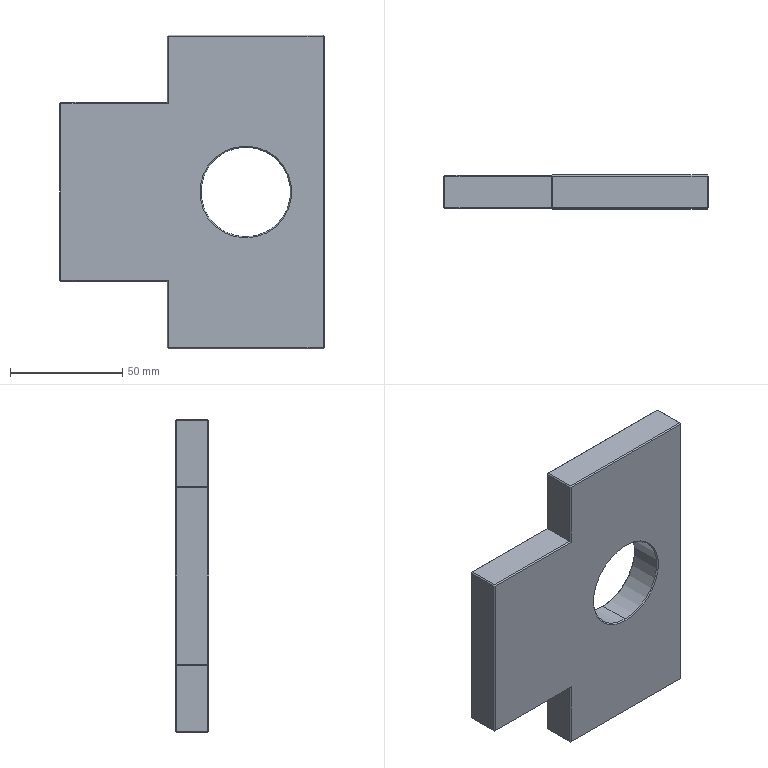Part | SolidWorks | features Chamfer 1, Extrusion 1 | 1 solid | 50 faces | box 118 x 15 x 140 mm | volume 185579 mm3 | plane 44 | cone 4 | cylinder 2 | commonest cylinder face diameters 40 x2
STEP:
#1=CARTESIAN_POINT('',(-35.,14.5,-20.));
#2=VERTEX_POINT('',#1);
#3=CARTESIAN_POINT('',(-35.,14.5,20.));
#4=VERTEX_POINT('',#3);
#5=CARTESIAN_POINT('',(-35.,14.5,0.));
#6=DIRECTION('',(0.,1.,0.));
#7=DIRECTION('',(0.,0.,-1.));
#8=AXIS2_PLACEMENT_3D('',#5,#6,#7);
#9=CIRCLE('',#8,20.);
#10=EDGE_CURVE('',#2,#4,#9,.T.);
#11=ORIENTED_EDGE('',*,*,#10,.F.);
#12=CARTESIAN_POINT('',(-35.,15.,-20.5));
#13=VERTEX_POINT('',#12);
#14=CARTESIAN_POINT('',(-35.,14.5,-20.));
#15=DIRECTION('',(0.,0.7071,-0.7071));
#16=VECTOR('',#15,1000.);
#17=LINE('',#14,#16);
#18=EDGE_CURVE('',#2,#13,#17,.T.);
#19=ORIENTED_EDGE('',*,*,#18,.T.);
#20=CARTESIAN_POINT('',(-35.,15.,20.5));
#21=VERTEX_POINT('',#20);
#22=CARTESIAN_POINT('',(-35.,15.,0.));
#23=DIRECTION('',(0.,-1.,0.));
#24=DIRECTION('',(0.,0.,-1.));
#25=AXIS2_PLACEMENT_3D('',#22,#23,#24);
#26=CIRCLE('',#25,20.5);
#27=EDGE_CURVE('',#21,#13,#26,.T.);
#28=ORIENTED_EDGE('',*,*,#27,.F.);
#29=CARTESIAN_POINT('',(-35.,14.5,20.));
#30=DIRECTION('',(0.,0.7071,0.7071));
#31=VECTOR('',#30,1000.);
#32=LINE('',#29,#31);
#33=EDGE_CURVE('',#4,#21,#32,.T.);
#34=ORIENTED_EDGE('',*,*,#33,.F.);
#35=EDGE_LOOP('',(#11,#19,#28,#34));
#36=FACE_OUTER_BOUND('',#35,.T.);
#37=CARTESIAN_POINT('',(-35.,14.5,0.));
#38=DIRECTION('',(0.,1.,0.));
#39=DIRECTION('',(0.,0.,1.));
#40=AXIS2_PLACEMENT_3D('',#37,#38,#39);
#41=CONICAL_SURFACE('',#40,20.,0.7854);
#42=ADVANCED_FACE('',(#36),#41,.F.);
#43=CARTESIAN_POINT('',(-35.,0.5,20.));
#44=VERTEX_POINT('',#43);
#45=CARTESIAN_POINT('',(-35.,0.5,-20.));
#46=VERTEX_POINT('',#45);
#47=CARTESIAN_POINT('',(-35.,0.5,0.));
#48=DIRECTION('',(0.,-1.,0.));
#49=DIRECTION('',(0.,0.,-1.));
#50=AXIS2_PLACEMENT_3D('',#47,#48,#49);
#51=CIRCLE('',#50,20.);
#52=EDGE_CURVE('',#44,#46,#51,.T.);
#53=ORIENTED_EDGE('',*,*,#52,.F.);
#54=CARTESIAN_POINT('',(-35.,0.,20.5));
#55=VERTEX_POINT('',#54);
#56=CARTESIAN_POINT('',(-35.,0.,20.5));
#57=DIRECTION('',(0.,-0.7071,0.7071));
#58=VECTOR('',#57,1000.);
#59=LINE('',#56,#58);
#60=EDGE_CURVE('',#44,#55,#59,.T.);
#61=ORIENTED_EDGE('',*,*,#60,.T.);
#62=CARTESIAN_POINT('',(-35.,0.,-20.5));
#63=VERTEX_POINT('',#62);
#64=CARTESIAN_POINT('',(-35.,0.,0.));
#65=DIRECTION('',(0.,1.,0.));
#66=DIRECTION('',(0.,0.,-1.));
#67=AXIS2_PLACEMENT_3D('',#64,#65,#66);
#68=CIRCLE('',#67,20.5);
#69=EDGE_CURVE('',#63,#55,#68,.T.);
#70=ORIENTED_EDGE('',*,*,#69,.F.);
#71=CARTESIAN_POINT('',(-35.,0.,-20.5));
#72=DIRECTION('',(0.,-0.7071,-0.7071));
#73=VECTOR('',#72,1000.);
#74=LINE('',#71,#73);
#75=EDGE_CURVE('',#46,#63,#74,.T.);
#76=ORIENTED_EDGE('',*,*,#75,.F.);
#77=EDGE_LOOP('',(#53,#61,#70,#76));
#78=FACE_OUTER_BOUND('',#77,.T.);
#79=CARTESIAN_POINT('',(-35.,0.,0.));
#80=DIRECTION('',(0.,-1.,0.));
#81=DIRECTION('',(0.,0.,-1.));
#82=AXIS2_PLACEMENT_3D('',#79,#80,#81);
#83=CONICAL_SURFACE('',#82,20.5,0.7854);
#84=ADVANCED_FACE('',(#78),#83,.F.);
#85=ORIENTED_EDGE('',*,*,#10,.T.);
#86=CARTESIAN_POINT('',(-35.,15.,20.));
#87=DIRECTION('',(0.,-1.,0.));
#88=VECTOR('',#87,1000.);
#89=LINE('',#86,#88);
#90=EDGE_CURVE('',#4,#44,#89,.T.);
#91=ORIENTED_EDGE('',*,*,#90,.T.);
#92=ORIENTED_EDGE('',*,*,#52,.T.);
#93=CARTESIAN_POINT('',(-35.,15.,-20.));
#94=DIRECTION('',(0.,-1.,0.));
#95=VECTOR('',#94,1000.);
#96=LINE('',#93,#95);
#97=EDGE_CURVE('',#2,#46,#96,.T.);
#98=ORIENTED_EDGE('',*,*,#97,.F.);
#99=EDGE_LOOP('',(#85,#91,#92,#98));
#100=FACE_OUTER_BOUND('',#99,.T.);
#101=CARTESIAN_POINT('',(-35.,15.,0.));
#102=DIRECTION('',(0.,-1.,0.));
#103=DIRECTION('',(0.,0.,-1.));
#104=AXIS2_PLACEMENT_3D('',#101,#102,#103);
#105=CYLINDRICAL_SURFACE('',#104,20.);
#106=ADVANCED_FACE('',(#100),#105,.F.);
#107=CARTESIAN_POINT('',(-117.5,15.,39.5));
#108=VERTEX_POINT('',#107);
#109=CARTESIAN_POINT('',(-69.5,15.,39.5));
#110=VERTEX_POINT('',#109);
#111=CARTESIAN_POINT('',(0.,15.,39.5));
#112=DIRECTION('',(1.,0.,0.));
#113=VECTOR('',#112,1000.);
#114=LINE('',#111,#113);
#115=EDGE_CURVE('',#108,#110,#114,.T.);
#116=ORIENTED_EDGE('',*,*,#115,.T.);
#117=CARTESIAN_POINT('',(-69.5,15.,69.5));
#118=VERTEX_POINT('',#117);
#119=CARTESIAN_POINT('',(-69.5,15.,0.));
#120=DIRECTION('',(0.,0.,1.));
#121=VECTOR('',#120,1000.);
#122=LINE('',#119,#121);
#123=EDGE_CURVE('',#110,#118,#122,.T.);
#124=ORIENTED_EDGE('',*,*,#123,.T.);
#125=CARTESIAN_POINT('',(-0.5,15.,69.5));
#126=VERTEX_POINT('',#125);
#127=CARTESIAN_POINT('',(0.,15.,69.5));
#128=DIRECTION('',(1.,0.,0.));
#129=VECTOR('',#128,1000.);
#130=LINE('',#127,#129);
#131=EDGE_CURVE('',#118,#126,#130,.T.);
#132=ORIENTED_EDGE('',*,*,#131,.T.);
#133=CARTESIAN_POINT('',(-0.5,15.,-69.5));
#134=VERTEX_POINT('',#133);
#135=CARTESIAN_POINT('',(-0.5,15.,0.));
#136=DIRECTION('',(0.,0.,-1.));
#137=VECTOR('',#136,1000.);
#138=LINE('',#135,#137);
#139=EDGE_CURVE('',#126,#134,#138,.T.);
#140=ORIENTED_EDGE('',*,*,#139,.T.);
#141=CARTESIAN_POINT('',(-69.5,15.,-69.5));
#142=VERTEX_POINT('',#141);
#143=CARTESIAN_POINT('',(0.,15.,-69.5));
#144=DIRECTION('',(-1.,0.,0.));
#145=VECTOR('',#144,1000.);
#146=LINE('',#143,#145);
#147=EDGE_CURVE('',#134,#142,#146,.T.);
#148=ORIENTED_EDGE('',*,*,#147,.T.);
#149=CARTESIAN_POINT('',(-69.5,15.,-39.5));
#150=VERTEX_POINT('',#149);
#151=CARTESIAN_POINT('',(-69.5,15.,0.));
#152=DIRECTION('',(0.,0.,1.));
#153=VECTOR('',#152,1000.);
#154=LINE('',#151,#153);
#155=EDGE_CURVE('',#142,#150,#154,.T.);
#156=ORIENTED_EDGE('',*,*,#155,.T.);
#157=CARTESIAN_POINT('',(-117.5,15.,-39.5));
#158=VERTEX_POINT('',#157);
#159=CARTESIAN_POINT('',(0.,15.,-39.5));
#160=DIRECTION('',(-1.,0.,0.));
#161=VECTOR('',#160,1000.);
#162=LINE('',#159,#161);
#163=EDGE_CURVE('',#150,#158,#162,.T.);
#164=ORIENTED_EDGE('',*,*,#163,.T.);
#165=CARTESIAN_POINT('',(-117.5,15.,0.));
#166=DIRECTION('',(0.,0.,1.));
#167=VECTOR('',#166,1000.);
#168=LINE('',#165,#167);
#169=EDGE_CURVE('',#158,#108,#168,.T.);
#170=ORIENTED_EDGE('',*,*,#169,.T.);
#171=EDGE_LOOP('',(#116,#124,#132,#140,#148,#156,#164,#170));
#172=FACE_OUTER_BOUND('',#171,.T.);
#173=ORIENTED_EDGE('',*,*,#27,.T.);
#174=CARTESIAN_POINT('',(-35.,15.,0.));
#175=DIRECTION('',(0.,-1.,0.));
#176=DIRECTION('',(0.,0.,-1.));
#177=AXIS2_PLACEMENT_3D('',#174,#175,#176);
#178=CIRCLE('',#177,20.5);
#179=EDGE_CURVE('',#13,#21,#178,.T.);
#180=ORIENTED_EDGE('',*,*,#179,.T.);
#181=EDGE_LOOP('',(#173,#180));
#182=FACE_BOUND('',#181,.T.);
#183=CARTESIAN_POINT('',(0.,15.,0.));
#184=DIRECTION('',(0.,-1.,0.));
#185=DIRECTION('',(0.,0.,-1.));
#186=AXIS2_PLACEMENT_3D('',#183,#184,#185);
#187=PLANE('',#186);
#188=ADVANCED_FACE('',(#172,#182),#187,.F.);
#189=ORIENTED_EDGE('',*,*,#69,.T.);
#190=CARTESIAN_POINT('',(-35.,0.,0.));
#191=DIRECTION('',(0.,1.,0.));
#192=DIRECTION('',(0.,0.,-1.));
#193=AXIS2_PLACEMENT_3D('',#190,#191,#192);
#194=CIRCLE('',#193,20.5);
#195=EDGE_CURVE('',#55,#63,#194,.T.);
#196=ORIENTED_EDGE('',*,*,#195,.T.);
#197=EDGE_LOOP('',(#189,#196));
#198=FACE_BOUND('',#197,.T.);
#199=CARTESIAN_POINT('',(-0.5,0.,69.5));
#200=VERTEX_POINT('',#199);
#201=CARTESIAN_POINT('',(-69.5,0.,69.5));
#202=VERTEX_POINT('',#201);
#203=CARTESIAN_POINT('',(-70.,0.,69.5));
#204=DIRECTION('',(-1.,0.,0.));
#205=VECTOR('',#204,1000.);
#206=LINE('',#203,#205);
#207=EDGE_CURVE('',#200,#202,#206,.T.);
#208=ORIENTED_EDGE('',*,*,#207,.T.);
#209=CARTESIAN_POINT('',(-69.5,0.,39.5));
#210=VERTEX_POINT('',#209);
#211=CARTESIAN_POINT('',(-69.5,0.,40.));
#212=DIRECTION('',(0.,0.,-1.));
#213=VECTOR('',#212,1000.);
#214=LINE('',#211,#213);
#215=EDGE_CURVE('',#202,#210,#214,.T.);
#216=ORIENTED_EDGE('',*,*,#215,.T.);
#217=CARTESIAN_POINT('',(-117.5,0.,39.5));
#218=VERTEX_POINT('',#217);
#219=CARTESIAN_POINT('',(-118.,0.,39.5));
#220=DIRECTION('',(-1.,0.,0.));
#221=VECTOR('',#220,1000.);
#222=LINE('',#219,#221);
#223=EDGE_CURVE('',#210,#218,#222,.T.);
#224=ORIENTED_EDGE('',*,*,#223,.T.);
#225=CARTESIAN_POINT('',(-117.5,0.,-39.5));
#226=VERTEX_POINT('',#225);
#227=CARTESIAN_POINT('',(-117.5,0.,-40.));
#228=DIRECTION('',(0.,0.,-1.));
#229=VECTOR('',#228,1000.);
#230=LINE('',#227,#229);
#231=EDGE_CURVE('',#218,#226,#230,.T.);
#232=ORIENTED_EDGE('',*,*,#231,.T.);
#233=CARTESIAN_POINT('',(-69.5,0.,-39.5));
#234=VERTEX_POINT('',#233);
#235=CARTESIAN_POINT('',(-70.,0.,-39.5));
#236=DIRECTION('',(1.,0.,0.));
#237=VECTOR('',#236,1000.);
#238=LINE('',#235,#237);
#239=EDGE_CURVE('',#226,#234,#238,.T.);
#240=ORIENTED_EDGE('',*,*,#239,.T.);
#241=CARTESIAN_POINT('',(-69.5,0.,-69.5));
#242=VERTEX_POINT('',#241);
#243=CARTESIAN_POINT('',(-69.5,0.,-70.));
#244=DIRECTION('',(0.,0.,-1.));
#245=VECTOR('',#244,1000.);
#246=LINE('',#243,#245);
#247=EDGE_CURVE('',#234,#242,#246,.T.);
#248=ORIENTED_EDGE('',*,*,#247,.T.);
#249=CARTESIAN_POINT('',(-0.5,0.,-69.5));
#250=VERTEX_POINT('',#249);
#251=CARTESIAN_POINT('',(0.,0.,-69.5));
#252=DIRECTION('',(1.,0.,0.));
#253=VECTOR('',#252,1000.);
#254=LINE('',#251,#253);
#255=EDGE_CURVE('',#242,#250,#254,.T.);
#256=ORIENTED_EDGE('',*,*,#255,.T.);
#257=CARTESIAN_POINT('',(-0.5,0.,70.));
#258=DIRECTION('',(0.,0.,1.));
#259=VECTOR('',#258,1000.);
#260=LINE('',#257,#259);
#261=EDGE_CURVE('',#250,#200,#260,.T.);
#262=ORIENTED_EDGE('',*,*,#261,.T.);
#263=EDGE_LOOP('',(#208,#216,#224,#232,#240,#248,#256,#262));
#264=FACE_OUTER_BOUND('',#263,.T.);
#265=CARTESIAN_POINT('',(0.,0.,0.));
#266=DIRECTION('',(0.,-1.,0.));
#267=DIRECTION('',(0.,0.,-1.));
#268=AXIS2_PLACEMENT_3D('',#265,#266,#267);
#269=PLANE('',#268);
#270=ADVANCED_FACE('',(#198,#264),#269,.T.);
#271=CARTESIAN_POINT('',(-0.5,0.5,70.));
#272=VERTEX_POINT('',#271);
#273=CARTESIAN_POINT('',(-0.5,14.5,70.));
#274=VERTEX_POINT('',#273);
#275=CARTESIAN_POINT('',(-0.5,15.,70.));
#276=DIRECTION('',(0.,1.,0.));
#277=VECTOR('',#276,1000.);
#278=LINE('',#275,#277);
#279=EDGE_CURVE('',#272,#274,#278,.T.);
#280=ORIENTED_EDGE('',*,*,#279,.T.);
#281=CARTESIAN_POINT('',(-69.5,14.5,70.));
#282=VERTEX_POINT('',#281);
#283=CARTESIAN_POINT('',(0.,14.5,70.));
#284=DIRECTION('',(-1.,0.,0.));
#285=VECTOR('',#284,1000.);
#286=LINE('',#283,#285);
#287=EDGE_CURVE('',#274,#282,#286,.T.);
#288=ORIENTED_EDGE('',*,*,#287,.T.);
#289=CARTESIAN_POINT('',(-69.5,0.5,70.));
#290=VERTEX_POINT('',#289);
#291=CARTESIAN_POINT('',(-69.5,15.,70.));
#292=DIRECTION('',(0.,-1.,0.));
#293=VECTOR('',#292,1000.);
#294=LINE('',#291,#293);
#295=EDGE_CURVE('',#282,#290,#294,.T.);
#296=ORIENTED_EDGE('',*,*,#295,.T.);
#297=CARTESIAN_POINT('',(0.,0.5,70.));
#298=DIRECTION('',(1.,0.,0.));
#299=VECTOR('',#298,1000.);
#300=LINE('',#297,#299);
#301=EDGE_CURVE('',#290,#272,#300,.T.);
#302=ORIENTED_EDGE('',*,*,#301,.T.);
#303=EDGE_LOOP('',(#280,#288,#296,#302));
#304=FACE_OUTER_BOUND('',#303,.T.);
#305=CARTESIAN_POINT('',(0.,15.,70.));
#306=DIRECTION('',(0.,0.,-1.));
#307=DIRECTION('',(-1.,0.,0.));
#308=AXIS2_PLACEMENT_3D('',#305,#306,#307);
#309=PLANE('',#308);
#310=ADVANCED_FACE('',(#304),#309,.F.);
#311=CARTESIAN_POINT('',(0.,0.5,-69.5));
#312=VERTEX_POINT('',#311);
#313=CARTESIAN_POINT('',(0.,14.5,-69.5));
#314=VERTEX_POINT('',#313);
#315=CARTESIAN_POINT('',(0.,15.,-69.5));
#316=DIRECTION('',(0.,1.,0.));
#317=VECTOR('',#316,1000.);
#318=LINE('',#315,#317);
#319=EDGE_CURVE('',#312,#314,#318,.T.);
#320=ORIENTED_EDGE('',*,*,#319,.T.);
#321=CARTESIAN_POINT('',(0.,14.5,69.5));
#322=VERTEX_POINT('',#321);
#323=CARTESIAN_POINT('',(0.,14.5,-70.));
#324=DIRECTION('',(0.,0.,1.));
#325=VECTOR('',#324,1000.);
#326=LINE('',#323,#325);
#327=EDGE_CURVE('',#314,#322,#326,.T.);
#328=ORIENTED_EDGE('',*,*,#327,.T.);
#329=CARTESIAN_POINT('',(0.,0.5,69.5));
#330=VERTEX_POINT('',#329);
#331=CARTESIAN_POINT('',(0.,15.,69.5));
#332=DIRECTION('',(0.,-1.,0.));
#333=VECTOR('',#332,1000.);
#334=LINE('',#331,#333);
#335=EDGE_CURVE('',#322,#330,#334,.T.);
#336=ORIENTED_EDGE('',*,*,#335,.T.);
#337=CARTESIAN_POINT('',(0.,0.5,-70.));
#338=DIRECTION('',(0.,0.,-1.));
#339=VECTOR('',#338,1000.);
#340=LINE('',#337,#339);
#341=EDGE_CURVE('',#330,#312,#340,.T.);
#342=ORIENTED_EDGE('',*,*,#341,.T.);
#343=EDGE_LOOP('',(#320,#328,#336,#342));
#344=FACE_OUTER_BOUND('',#343,.T.);
#345=CARTESIAN_POINT('',(0.,15.,-70.));
#346=DIRECTION('',(-1.,0.,0.));
#347=DIRECTION('',(0.,0.,1.));
#348=AXIS2_PLACEMENT_3D('',#345,#346,#347);
#349=PLANE('',#348);
#350=ADVANCED_FACE('',(#344),#349,.F.);
#351=CARTESIAN_POINT('',(-69.5,14.5,-70.));
#352=VERTEX_POINT('',#351);
#353=CARTESIAN_POINT('',(-0.5,14.5,-70.));
#354=VERTEX_POINT('',#353);
#355=CARTESIAN_POINT('',(-70.,14.5,-70.));
#356=DIRECTION('',(1.,0.,0.));
#357=VECTOR('',#356,1000.);
#358=LINE('',#355,#357);
#359=EDGE_CURVE('',#352,#354,#358,.T.);
#360=ORIENTED_EDGE('',*,*,#359,.T.);
#361=CARTESIAN_POINT('',(-0.5,0.5,-70.));
#362=VERTEX_POINT('',#361);
#363=CARTESIAN_POINT('',(-0.5,15.,-70.));
#364=DIRECTION('',(0.,-1.,0.));
#365=VECTOR('',#364,1000.);
#366=LINE('',#363,#365);
#367=EDGE_CURVE('',#354,#362,#366,.T.);
#368=ORIENTED_EDGE('',*,*,#367,.T.);
#369=CARTESIAN_POINT('',(-69.5,0.5,-70.));
#370=VERTEX_POINT('',#369);
#371=CARTESIAN_POINT('',(-70.,0.5,-70.));
#372=DIRECTION('',(-1.,0.,0.));
#373=VECTOR('',#372,1000.);
#374=LINE('',#371,#373);
#375=EDGE_CURVE('',#362,#370,#374,.T.);
#376=ORIENTED_EDGE('',*,*,#375,.T.);
#377=CARTESIAN_POINT('',(-69.5,15.,-70.));
#378=DIRECTION('',(0.,1.,0.));
#379=VECTOR('',#378,1000.);
#380=LINE('',#377,#379);
#381=EDGE_CURVE('',#370,#352,#380,.T.);
#382=ORIENTED_EDGE('',*,*,#381,.T.);
#383=EDGE_LOOP('',(#360,#368,#376,#382));
#384=FACE_OUTER_BOUND('',#383,.T.);
#385=CARTESIAN_POINT('',(-70.,15.,-70.));
#386=DIRECTION('',(0.,0.,1.));
#387=DIRECTION('',(1.,0.,0.));
#388=AXIS2_PLACEMENT_3D('',#385,#386,#387);
#389=PLANE('',#388);
#390=ADVANCED_FACE('',(#384),#389,.F.);
#391=CARTESIAN_POINT('',(-70.,14.5,-40.));
#392=VERTEX_POINT('',#391);
#393=CARTESIAN_POINT('',(-70.,0.5,-40.));
#394=VERTEX_POINT('',#393);
#395=CARTESIAN_POINT('',(-70.,15.,-40.));
#396=DIRECTION('',(0.,-1.,0.));
#397=VECTOR('',#396,1000.);
#398=LINE('',#395,#397);
#399=EDGE_CURVE('',#392,#394,#398,.T.);
#400=ORIENTED_EDGE('',*,*,#399,.F.);
#401=CARTESIAN_POINT('',(-70.,14.5,-69.5));
#402=VERTEX_POINT('',#401);
#403=CARTESIAN_POINT('',(-70.,14.5,-40.));
#404=DIRECTION('',(0.,0.,-1.));
#405=VECTOR('',#404,1000.);
#406=LINE('',#403,#405);
#407=EDGE_CURVE('',#392,#402,#406,.T.);
#408=ORIENTED_EDGE('',*,*,#407,.T.);
#409=CARTESIAN_POINT('',(-70.,0.5,-69.5));
#410=VERTEX_POINT('',#409);
#411=CARTESIAN_POINT('',(-70.,15.,-69.5));
#412=DIRECTION('',(0.,-1.,0.));
#413=VECTOR('',#412,1000.);
#414=LINE('',#411,#413);
#415=EDGE_CURVE('',#402,#410,#414,.T.);
#416=ORIENTED_EDGE('',*,*,#415,.T.);
#417=CARTESIAN_POINT('',(-70.,0.5,-40.));
#418=DIRECTION('',(0.,0.,1.));
#419=VECTOR('',#418,1000.);
#420=LINE('',#417,#419);
#421=EDGE_CURVE('',#410,#394,#420,.T.);
#422=ORIENTED_EDGE('',*,*,#421,.T.);
#423=EDGE_LOOP('',(#400,#408,#416,#422));
#424=FACE_OUTER_BOUND('',#423,.T.);
#425=CARTESIAN_POINT('',(-70.,15.,-40.));
#426=DIRECTION('',(1.,0.,0.));
#427=DIRECTION('',(0.,0.,-1.));
#428=AXIS2_PLACEMENT_3D('',#425,#426,#427);
#429=PLANE('',#428);
#430=ADVANCED_FACE('',(#424),#429,.F.);
#431=CARTESIAN_POINT('',(-117.5,0.5,-40.));
#432=VERTEX_POINT('',#431);
#433=CARTESIAN_POINT('',(-117.5,14.5,-40.));
#434=VERTEX_POINT('',#433);
#435=CARTESIAN_POINT('',(-117.5,15.,-40.));
#436=DIRECTION('',(0.,1.,0.));
#437=VECTOR('',#436,1000.);
#438=LINE('',#435,#437);
#439=EDGE_CURVE('',#432,#434,#438,.T.);
#440=ORIENTED_EDGE('',*,*,#439,.T.);
#441=CARTESIAN_POINT('',(-118.,14.5,-40.));
#442=DIRECTION('',(1.,0.,0.));
#443=VECTOR('',#442,1000.);
#444=LINE('',#441,#443);
#445=EDGE_CURVE('',#434,#392,#444,.T.);
#446=ORIENTED_EDGE('',*,*,#445,.T.);
#447=ORIENTED_EDGE('',*,*,#399,.T.);
#448=CARTESIAN_POINT('',(-118.,0.5,-40.));
#449=DIRECTION('',(-1.,0.,0.));
#450=VECTOR('',#449,1000.);
#451=LINE('',#448,#450);
#452=EDGE_CURVE('',#394,#432,#451,.T.);
#453=ORIENTED_EDGE('',*,*,#452,.T.);
#454=EDGE_LOOP('',(#440,#446,#447,#453));
#455=FACE_OUTER_BOUND('',#454,.T.);
#456=CARTESIAN_POINT('',(-118.,15.,-40.));
#457=DIRECTION('',(0.,0.,1.));
#458=DIRECTION('',(1.,0.,0.));
#459=AXIS2_PLACEMENT_3D('',#456,#457,#458);
#460=PLANE('',#459);
#461=ADVANCED_FACE('',(#455),#460,.F.);
#462=CARTESIAN_POINT('',(-118.,0.5,39.5));
#463=VERTEX_POINT('',#462);
#464=CARTESIAN_POINT('',(-118.,14.5,39.5));
#465=VERTEX_POINT('',#464);
#466=CARTESIAN_POINT('',(-118.,15.,39.5));
#467=DIRECTION('',(0.,1.,0.));
#468=VECTOR('',#467,1000.);
#469=LINE('',#466,#468);
#470=EDGE_CURVE('',#463,#465,#469,.T.);
#471=ORIENTED_EDGE('',*,*,#470,.T.);
#472=CARTESIAN_POINT('',(-118.,14.5,-39.5));
#473=VERTEX_POINT('',#472);
#474=CARTESIAN_POINT('',(-118.,14.5,40.));
#475=DIRECTION('',(0.,0.,-1.));
#476=VECTOR('',#475,1000.);
#477=LINE('',#474,#476);
#478=EDGE_CURVE('',#465,#473,#477,.T.);
#479=ORIENTED_EDGE('',*,*,#478,.T.);
#480=CARTESIAN_POINT('',(-118.,0.5,-39.5));
#481=VERTEX_POINT('',#480);
#482=CARTESIAN_POINT('',(-118.,15.,-39.5));
#483=DIRECTION('',(0.,-1.,0.));
#484=VECTOR('',#483,1000.);
#485=LINE('',#482,#484);
#486=EDGE_CURVE('',#473,#481,#485,.T.);
#487=ORIENTED_EDGE('',*,*,#486,.T.);
#488=CARTESIAN_POINT('',(-118.,0.5,40.));
#489=DIRECTION('',(0.,0.,1.));
#490=VECTOR('',#489,1000.);
#491=LINE('',#488,#490);
#492=EDGE_CURVE('',#481,#463,#491,.T.);
#493=ORIENTED_EDGE('',*,*,#492,.T.);
#494=EDGE_LOOP('',(#471,#479,#487,#493));
#495=FACE_OUTER_BOUND('',#494,.T.);
#496=CARTESIAN_POINT('',(-118.,15.,40.));
#497=DIRECTION('',(1.,0.,0.));
#498=DIRECTION('',(0.,0.,-1.));
#499=AXIS2_PLACEMENT_3D('',#496,#497,#498);
#500=PLANE('',#499);
#501=ADVANCED_FACE('',(#495),#500,.F.);
#502=CARTESIAN_POINT('',(-70.,14.5,40.));
#503=VERTEX_POINT('',#502);
#504=CARTESIAN_POINT('',(-70.,0.5,40.));
#505=VERTEX_POINT('',#504);
#506=CARTESIAN_POINT('',(-70.,15.,40.));
#507=DIRECTION('',(0.,-1.,0.));
#508=VECTOR('',#507,1000.);
#509=LINE('',#506,#508);
#510=EDGE_CURVE('',#503,#505,#509,.T.);
#511=ORIENTED_EDGE('',*,*,#510,.F.);
#512=CARTESIAN_POINT('',(-117.5,14.5,40.));
#513=VERTEX_POINT('',#512);
#514=CARTESIAN_POINT('',(-70.,14.5,40.));
#515=DIRECTION('',(-1.,0.,0.));
#516=VECTOR('',#515,1000.);
#517=LINE('',#514,#516);
#518=EDGE_CURVE('',#503,#513,#517,.T.);
#519=ORIENTED_EDGE('',*,*,#518,.T.);
#520=CARTESIAN_POINT('',(-117.5,0.5,40.));
#521=VERTEX_POINT('',#520);
#522=CARTESIAN_POINT('',(-117.5,15.,40.));
#523=DIRECTION('',(0.,-1.,0.));
#524=VECTOR('',#523,1000.);
#525=LINE('',#522,#524);
#526=EDGE_CURVE('',#513,#521,#525,.T.);
#527=ORIENTED_EDGE('',*,*,#526,.T.);
#528=CARTESIAN_POINT('',(-70.,0.5,40.));
#529=DIRECTION('',(1.,0.,0.));
#530=VECTOR('',#529,1000.);
#531=LINE('',#528,#530);
#532=EDGE_CURVE('',#521,#505,#531,.T.);
#533=ORIENTED_EDGE('',*,*,#532,.T.);
#534=EDGE_LOOP('',(#511,#519,#527,#533));
#535=FACE_OUTER_BOUND('',#534,.T.);
#536=CARTESIAN_POINT('',(-70.,15.,40.));
#537=DIRECTION('',(0.,0.,-1.));
#538=DIRECTION('',(-1.,0.,0.));
#539=AXIS2_PLACEMENT_3D('',#536,#537,#538);
#540=PLANE('',#539);
#541=ADVANCED_FACE('',(#535),#540,.F.);
#542=CARTESIAN_POINT('',(-70.,0.5,69.5));
#543=VERTEX_POINT('',#542);
#544=CARTESIAN_POINT('',(-70.,14.5,69.5));
#545=VERTEX_POINT('',#544);
#546=CARTESIAN_POINT('',(-70.,15.,69.5));
#547=DIRECTION('',(0.,1.,0.));
#548=VECTOR('',#547,1000.);
#549=LINE('',#546,#548);
#550=EDGE_CURVE('',#543,#545,#549,.T.);
#551=ORIENTED_EDGE('',*,*,#550,.T.);
#552=CARTESIAN_POINT('',(-70.,14.5,70.));
#553=DIRECTION('',(0.,0.,-1.));
#554=VECTOR('',#553,1000.);
#555=LINE('',#552,#554);
#556=EDGE_CURVE('',#545,#503,#555,.T.);
#557=ORIENTED_EDGE('',*,*,#556,.T.);
#558=ORIENTED_EDGE('',*,*,#510,.T.);
#559=CARTESIAN_POINT('',(-70.,0.5,70.));
#560=DIRECTION('',(0.,0.,1.));
#561=VECTOR('',#560,1000.);
#562=LINE('',#559,#561);
#563=EDGE_CURVE('',#505,#543,#562,.T.);
#564=ORIENTED_EDGE('',*,*,#563,.T.);
#565=EDGE_LOOP('',(#551,#557,#558,#564));
#566=FACE_OUTER_BOUND('',#565,.T.);
#567=CARTESIAN_POINT('',(-70.,15.,70.));
#568=DIRECTION('',(1.,0.,0.));
#569=DIRECTION('',(0.,0.,-1.));
#570=AXIS2_PLACEMENT_3D('',#567,#568,#569);
#571=PLANE('',#570);
#572=ADVANCED_FACE('',(#566),#571,.F.);
#573=ORIENTED_EDGE('',*,*,#90,.F.);
#574=CARTESIAN_POINT('',(-35.,14.5,0.));
#575=DIRECTION('',(0.,1.,0.));
#576=DIRECTION('',(0.,0.,-1.));
#577=AXIS2_PLACEMENT_3D('',#574,#575,#576);
#578=CIRCLE('',#577,20.);
#579=EDGE_CURVE('',#4,#2,#578,.T.);
#580=ORIENTED_EDGE('',*,*,#579,.T.);
#581=ORIENTED_EDGE('',*,*,#97,.T.);
#582=CARTESIAN_POINT('',(-35.,0.5,0.));
#583=DIRECTION('',(0.,-1.,0.));
#584=DIRECTION('',(0.,0.,-1.));
#585=AXIS2_PLACEMENT_3D('',#582,#583,#584);
#586=CIRCLE('',#585,20.);
#587=EDGE_CURVE('',#46,#44,#586,.T.);
#588=ORIENTED_EDGE('',*,*,#587,.T.);
#589=EDGE_LOOP('',(#573,#580,#581,#588));
#590=FACE_OUTER_BOUND('',#589,.T.);
#591=CARTESIAN_POINT('',(-35.,15.,0.));
#592=DIRECTION('',(0.,-1.,0.));
#593=DIRECTION('',(0.,0.,-1.));
#594=AXIS2_PLACEMENT_3D('',#591,#592,#593);
#595=CYLINDRICAL_SURFACE('',#594,20.);
#596=ADVANCED_FACE('',(#590),#595,.F.);
#597=ORIENTED_EDGE('',*,*,#60,.F.);
#598=ORIENTED_EDGE('',*,*,#587,.F.);
#599=ORIENTED_EDGE('',*,*,#75,.T.);
#600=ORIENTED_EDGE('',*,*,#195,.F.);
#601=EDGE_LOOP('',(#597,#598,#599,#600));
#602=FACE_OUTER_BOUND('',#601,.T.);
#603=CARTESIAN_POINT('',(-35.,0.,0.));
#604=DIRECTION('',(0.,-1.,0.));
#605=DIRECTION('',(0.,0.,-1.));
#606=AXIS2_PLACEMENT_3D('',#603,#604,#605);
#607=CONICAL_SURFACE('',#606,20.5,0.7854);
#608=ADVANCED_FACE('',(#602),#607,.F.);
#609=CARTESIAN_POINT('',(-118.,14.5,39.5));
#610=DIRECTION('',(0.7071,0.,0.7071));
#611=VECTOR('',#610,1000.);
#612=LINE('',#609,#611);
#613=EDGE_CURVE('',#465,#513,#612,.T.);
#614=ORIENTED_EDGE('',*,*,#613,.F.);
#615=ORIENTED_EDGE('',*,*,#470,.F.);
#616=CARTESIAN_POINT('',(-117.5,0.5,40.));
#617=DIRECTION('',(-0.7071,0.,-0.7071));
#618=VECTOR('',#617,1000.);
#619=LINE('',#616,#618);
#620=EDGE_CURVE('',#521,#463,#619,.T.);
#621=ORIENTED_EDGE('',*,*,#620,.F.);
#622=ORIENTED_EDGE('',*,*,#526,.F.);
#623=EDGE_LOOP('',(#614,#615,#621,#622));
#624=FACE_OUTER_BOUND('',#623,.T.);
#625=CARTESIAN_POINT('',(-117.5,15.,40.));
#626=DIRECTION('',(0.7071,0.,-0.7071));
#627=DIRECTION('',(0.,-1.,0.));
#628=AXIS2_PLACEMENT_3D('',#625,#626,#627);
#629=PLANE('',#628);
#630=ADVANCED_FACE('',(#624),#629,.F.);
#631=CARTESIAN_POINT('',(-118.,14.5,39.5));
#632=DIRECTION('',(0.7071,0.7071,0.));
#633=VECTOR('',#632,1000.);
#634=LINE('',#631,#633);
#635=EDGE_CURVE('',#465,#108,#634,.T.);
#636=ORIENTED_EDGE('',*,*,#635,.F.);
#637=ORIENTED_EDGE('',*,*,#613,.T.);
#638=CARTESIAN_POINT('',(-117.5,14.75,39.75));
#639=DIRECTION('',(0.,-0.7071,0.7071));
#640=VECTOR('',#639,1000.);
#641=LINE('',#638,#640);
#642=EDGE_CURVE('',#108,#513,#641,.T.);
#643=ORIENTED_EDGE('',*,*,#642,.F.);
#644=EDGE_LOOP('',(#636,#637,#643));
#645=FACE_OUTER_BOUND('',#644,.T.);
#646=CARTESIAN_POINT('',(-118.,14.5,39.5));
#647=DIRECTION('',(-0.5774,0.5774,0.5774));
#648=DIRECTION('',(0.7071,0.,0.7071));
#649=AXIS2_PLACEMENT_3D('',#646,#647,#648);
#650=PLANE('',#649);
#651=ADVANCED_FACE('',(#645),#650,.T.);
#652=CARTESIAN_POINT('',(-117.5,0.5,40.));
#653=DIRECTION('',(0.,-0.7071,-0.7071));
#654=VECTOR('',#653,1000.);
#655=LINE('',#652,#654);
#656=EDGE_CURVE('',#521,#218,#655,.T.);
#657=ORIENTED_EDGE('',*,*,#656,.F.);
#658=ORIENTED_EDGE('',*,*,#620,.T.);
#659=CARTESIAN_POINT('',(-117.75,0.25,39.5));
#660=DIRECTION('',(-0.7071,0.7071,0.));
#661=VECTOR('',#660,1000.);
#662=LINE('',#659,#661);
#663=EDGE_CURVE('',#218,#463,#662,.T.);
#664=ORIENTED_EDGE('',*,*,#663,.F.);
#665=EDGE_LOOP('',(#657,#658,#664));
#666=FACE_OUTER_BOUND('',#665,.T.);
#667=CARTESIAN_POINT('',(-117.5,0.5,40.));
#668=DIRECTION('',(-0.5774,-0.5774,0.5774));
#669=DIRECTION('',(0.7071,0.,0.7071));
#670=AXIS2_PLACEMENT_3D('',#667,#668,#669);
#671=PLANE('',#670);
#672=ADVANCED_FACE('',(#666),#671,.T.);
#673=ORIENTED_EDGE('',*,*,#642,.T.);
#674=ORIENTED_EDGE('',*,*,#518,.F.);
#675=CARTESIAN_POINT('',(-56.333,28.167,26.333));
#676=DIRECTION('',(-0.5774,-0.5774,0.5774));
#677=VECTOR('',#676,1000.);
#678=LINE('',#675,#677);
#679=EDGE_CURVE('',#110,#503,#678,.T.);
#680=ORIENTED_EDGE('',*,*,#679,.F.);
#681=ORIENTED_EDGE('',*,*,#115,.F.);
#682=EDGE_LOOP('',(#673,#674,#680,#681));
#683=FACE_OUTER_BOUND('',#682,.T.);
#684=CARTESIAN_POINT('',(0.,15.,39.5));
#685=DIRECTION('',(0.,-0.7071,-0.7071));
#686=DIRECTION('',(1.,0.,0.));
#687=AXIS2_PLACEMENT_3D('',#684,#685,#686);
#688=PLANE('',#687);
#689=ADVANCED_FACE('',(#683),#688,.F.);
#690=ORIENTED_EDGE('',*,*,#635,.T.);
#691=ORIENTED_EDGE('',*,*,#169,.F.);
#692=CARTESIAN_POINT('',(-117.75,14.75,-39.5));
#693=DIRECTION('',(0.7071,0.7071,0.));
#694=VECTOR('',#693,1000.);
#695=LINE('',#692,#694);
#696=EDGE_CURVE('',#473,#158,#695,.T.);
#697=ORIENTED_EDGE('',*,*,#696,.F.);
#698=ORIENTED_EDGE('',*,*,#478,.F.);
#699=EDGE_LOOP('',(#690,#691,#697,#698));
#700=FACE_OUTER_BOUND('',#699,.T.);
#701=CARTESIAN_POINT('',(-117.5,15.,0.));
#702=DIRECTION('',(0.7071,-0.7071,0.));
#703=DIRECTION('',(0.,0.,1.));
#704=AXIS2_PLACEMENT_3D('',#701,#702,#703);
#705=PLANE('',#704);
#706=ADVANCED_FACE('',(#700),#705,.F.);
#707=CARTESIAN_POINT('',(-118.,0.5,-39.5));
#708=DIRECTION('',(0.7071,0.,-0.7071));
#709=VECTOR('',#708,1000.);
#710=LINE('',#707,#709);
#711=EDGE_CURVE('',#481,#432,#710,.T.);
#712=ORIENTED_EDGE('',*,*,#711,.F.);
#713=ORIENTED_EDGE('',*,*,#486,.F.);
#714=CARTESIAN_POINT('',(-117.5,14.5,-40.));
#715=DIRECTION('',(-0.7071,0.,0.7071));
#716=VECTOR('',#715,1000.);
#717=LINE('',#714,#716);
#718=EDGE_CURVE('',#434,#473,#717,.T.);
#719=ORIENTED_EDGE('',*,*,#718,.F.);
#720=ORIENTED_EDGE('',*,*,#439,.F.);
#721=EDGE_LOOP('',(#712,#713,#719,#720));
#722=FACE_OUTER_BOUND('',#721,.T.);
#723=CARTESIAN_POINT('',(-118.,15.,-39.5));
#724=DIRECTION('',(0.7071,0.,0.7071));
#725=DIRECTION('',(0.,-1.,0.));
#726=AXIS2_PLACEMENT_3D('',#723,#724,#725);
#727=PLANE('',#726);
#728=ADVANCED_FACE('',(#722),#727,.F.);
#729=ORIENTED_EDGE('',*,*,#663,.T.);
#730=ORIENTED_EDGE('',*,*,#492,.F.);
#731=CARTESIAN_POINT('',(-118.,0.5,-39.5));
#732=DIRECTION('',(-0.7071,0.7071,0.));
#733=VECTOR('',#732,1000.);
#734=LINE('',#731,#733);
#735=EDGE_CURVE('',#226,#481,#734,.T.);
#736=ORIENTED_EDGE('',*,*,#735,.F.);
#737=ORIENTED_EDGE('',*,*,#231,.F.);
#738=EDGE_LOOP('',(#729,#730,#736,#737));
#739=FACE_OUTER_BOUND('',#738,.T.);
#740=CARTESIAN_POINT('',(-118.,0.5,40.));
#741=DIRECTION('',(-0.7071,-0.7071,0.));
#742=DIRECTION('',(0.,0.,-1.));
#743=AXIS2_PLACEMENT_3D('',#740,#741,#742);
#744=PLANE('',#743);
#745=ADVANCED_FACE('',(#739),#744,.T.);
#746=ORIENTED_EDGE('',*,*,#656,.T.);
#747=ORIENTED_EDGE('',*,*,#223,.F.);
#748=CARTESIAN_POINT('',(-80.,10.5,50.));
#749=DIRECTION('',(0.5774,-0.5774,-0.5774));
#750=VECTOR('',#749,1000.);
#751=LINE('',#748,#750);
#752=EDGE_CURVE('',#505,#210,#751,.T.);
#753=ORIENTED_EDGE('',*,*,#752,.F.);
#754=ORIENTED_EDGE('',*,*,#532,.F.);
#755=EDGE_LOOP('',(#746,#747,#753,#754));
#756=FACE_OUTER_BOUND('',#755,.T.);
#757=CARTESIAN_POINT('',(-70.,0.5,40.));
#758=DIRECTION('',(0.,-0.7071,0.7071));
#759=DIRECTION('',(-1.,0.,0.));
#760=AXIS2_PLACEMENT_3D('',#757,#758,#759);
#761=PLANE('',#760);
#762=ADVANCED_FACE('',(#756),#761,.T.);
#763=ORIENTED_EDGE('',*,*,#679,.T.);
#764=ORIENTED_EDGE('',*,*,#556,.F.);
#765=CARTESIAN_POINT('',(-70.,14.5,69.5));
#766=DIRECTION('',(-0.7071,-0.7071,0.));
#767=VECTOR('',#766,1000.);
#768=LINE('',#765,#767);
#769=EDGE_CURVE('',#118,#545,#768,.T.);
#770=ORIENTED_EDGE('',*,*,#769,.F.);
#771=ORIENTED_EDGE('',*,*,#123,.F.);
#772=EDGE_LOOP('',(#763,#764,#770,#771));
#773=FACE_OUTER_BOUND('',#772,.T.);
#774=CARTESIAN_POINT('',(-69.5,15.,0.));
#775=DIRECTION('',(0.7071,-0.7071,0.));
#776=DIRECTION('',(0.,0.,1.));
#777=AXIS2_PLACEMENT_3D('',#774,#775,#776);
#778=PLANE('',#777);
#779=ADVANCED_FACE('',(#773),#778,.F.);
#780=ORIENTED_EDGE('',*,*,#718,.T.);
#781=ORIENTED_EDGE('',*,*,#696,.T.);
#782=CARTESIAN_POINT('',(-117.5,14.5,-40.));
#783=DIRECTION('',(0.,0.7071,0.7071));
#784=VECTOR('',#783,1000.);
#785=LINE('',#782,#784);
#786=EDGE_CURVE('',#434,#158,#785,.T.);
#787=ORIENTED_EDGE('',*,*,#786,.F.);
#788=EDGE_LOOP('',(#780,#781,#787));
#789=FACE_OUTER_BOUND('',#788,.T.);
#790=CARTESIAN_POINT('',(-117.5,14.5,-40.));
#791=DIRECTION('',(-0.5774,0.5774,-0.5774));
#792=DIRECTION('',(-0.7071,0.,0.7071));
#793=AXIS2_PLACEMENT_3D('',#790,#791,#792);
#794=PLANE('',#793);
#795=ADVANCED_FACE('',(#789),#794,.T.);
#796=ORIENTED_EDGE('',*,*,#735,.T.);
#797=ORIENTED_EDGE('',*,*,#711,.T.);
#798=CARTESIAN_POINT('',(-117.5,0.25,-39.75));
#799=DIRECTION('',(0.,0.7071,-0.7071));
#800=VECTOR('',#799,1000.);
#801=LINE('',#798,#800);
#802=EDGE_CURVE('',#226,#432,#801,.T.);
#803=ORIENTED_EDGE('',*,*,#802,.F.);
#804=EDGE_LOOP('',(#796,#797,#803));
#805=FACE_OUTER_BOUND('',#804,.T.);
#806=CARTESIAN_POINT('',(-118.,0.5,-39.5));
#807=DIRECTION('',(-0.5774,-0.5774,-0.5774));
#808=DIRECTION('',(-0.7071,0.,0.7071));
#809=AXIS2_PLACEMENT_3D('',#806,#807,#808);
#810=PLANE('',#809);
#811=ADVANCED_FACE('',(#805),#810,.T.);
#812=ORIENTED_EDGE('',*,*,#752,.T.);
#813=ORIENTED_EDGE('',*,*,#215,.F.);
#814=CARTESIAN_POINT('',(-69.75,0.25,69.5));
#815=DIRECTION('',(0.7071,-0.7071,0.));
#816=VECTOR('',#815,1000.);
#817=LINE('',#814,#816);
#818=EDGE_CURVE('',#543,#202,#817,.T.);
#819=ORIENTED_EDGE('',*,*,#818,.F.);
#820=ORIENTED_EDGE('',*,*,#563,.F.);
#821=EDGE_LOOP('',(#812,#813,#819,#820));
#822=FACE_OUTER_BOUND('',#821,.T.);
#823=CARTESIAN_POINT('',(-70.,0.5,70.));
#824=DIRECTION('',(-0.7071,-0.7071,0.));
#825=DIRECTION('',(0.,0.,-1.));
#826=AXIS2_PLACEMENT_3D('',#823,#824,#825);
#827=PLANE('',#826);
#828=ADVANCED_FACE('',(#822),#827,.T.);
#829=CARTESIAN_POINT('',(-70.,14.5,69.5));
#830=DIRECTION('',(0.7071,0.,0.7071));
#831=VECTOR('',#830,1000.);
#832=LINE('',#829,#831);
#833=EDGE_CURVE('',#545,#282,#832,.T.);
#834=ORIENTED_EDGE('',*,*,#833,.F.);
#835=ORIENTED_EDGE('',*,*,#550,.F.);
#836=CARTESIAN_POINT('',(-69.5,0.5,70.));
#837=DIRECTION('',(-0.7071,0.,-0.7071));
#838=VECTOR('',#837,1000.);
#839=LINE('',#836,#838);
#840=EDGE_CURVE('',#290,#543,#839,.T.);
#841=ORIENTED_EDGE('',*,*,#840,.F.);
#842=ORIENTED_EDGE('',*,*,#295,.F.);
#843=EDGE_LOOP('',(#834,#835,#841,#842));
#844=FACE_OUTER_BOUND('',#843,.T.);
#845=CARTESIAN_POINT('',(-69.5,15.,70.));
#846=DIRECTION('',(0.7071,0.,-0.7071));
#847=DIRECTION('',(0.,-1.,0.));
#848=AXIS2_PLACEMENT_3D('',#845,#846,#847);
#849=PLANE('',#848);
#850=ADVANCED_FACE('',(#844),#849,.F.);
#851=ORIENTED_EDGE('',*,*,#769,.T.);
#852=ORIENTED_EDGE('',*,*,#833,.T.);
#853=CARTESIAN_POINT('',(-69.5,14.75,69.75));
#854=DIRECTION('',(0.,-0.7071,0.7071));
#855=VECTOR('',#854,1000.);
#856=LINE('',#853,#855);
#857=EDGE_CURVE('',#118,#282,#856,.T.);
#858=ORIENTED_EDGE('',*,*,#857,.F.);
#859=EDGE_LOOP('',(#851,#852,#858));
#860=FACE_OUTER_BOUND('',#859,.T.);
#861=CARTESIAN_POINT('',(-70.,14.5,69.5));
#862=DIRECTION('',(-0.5774,0.5774,0.5774));
#863=DIRECTION('',(0.7071,0.,0.7071));
#864=AXIS2_PLACEMENT_3D('',#861,#862,#863);
#865=PLANE('',#864);
#866=ADVANCED_FACE('',(#860),#865,.T.);
#867=ORIENTED_EDGE('',*,*,#786,.T.);
#868=ORIENTED_EDGE('',*,*,#163,.F.);
#869=CARTESIAN_POINT('',(-46.333,38.167,-16.333));
#870=DIRECTION('',(0.5774,0.5774,0.5774));
#871=VECTOR('',#870,1000.);
#872=LINE('',#869,#871);
#873=EDGE_CURVE('',#392,#150,#872,.T.);
#874=ORIENTED_EDGE('',*,*,#873,.F.);
#875=ORIENTED_EDGE('',*,*,#445,.F.);
#876=EDGE_LOOP('',(#867,#868,#874,#875));
#877=FACE_OUTER_BOUND('',#876,.T.);
#878=CARTESIAN_POINT('',(0.,15.,-39.5));
#879=DIRECTION('',(0.,-0.7071,0.7071));
#880=DIRECTION('',(-1.,0.,0.));
#881=AXIS2_PLACEMENT_3D('',#878,#879,#880);
#882=PLANE('',#881);
#883=ADVANCED_FACE('',(#877),#882,.F.);
#884=ORIENTED_EDGE('',*,*,#802,.T.);
#885=ORIENTED_EDGE('',*,*,#452,.F.);
#886=CARTESIAN_POINT('',(-86.,16.5,-56.));
#887=DIRECTION('',(-0.5774,0.5774,-0.5774));
#888=VECTOR('',#887,1000.);
#889=LINE('',#886,#888);
#890=EDGE_CURVE('',#234,#394,#889,.T.);
#891=ORIENTED_EDGE('',*,*,#890,.F.);
#892=ORIENTED_EDGE('',*,*,#239,.F.);
#893=EDGE_LOOP('',(#884,#885,#891,#892));
#894=FACE_OUTER_BOUND('',#893,.T.);
#895=CARTESIAN_POINT('',(-118.,0.5,-40.));
#896=DIRECTION('',(0.,-0.7071,-0.7071));
#897=DIRECTION('',(1.,0.,0.));
#898=AXIS2_PLACEMENT_3D('',#895,#896,#897);
#899=PLANE('',#898);
#900=ADVANCED_FACE('',(#894),#899,.T.);
#901=ORIENTED_EDGE('',*,*,#840,.T.);
#902=ORIENTED_EDGE('',*,*,#818,.T.);
#903=CARTESIAN_POINT('',(-69.5,0.5,70.));
#904=DIRECTION('',(0.,-0.7071,-0.7071));
#905=VECTOR('',#904,1000.);
#906=LINE('',#903,#905);
#907=EDGE_CURVE('',#290,#202,#906,.T.);
#908=ORIENTED_EDGE('',*,*,#907,.F.);
#909=EDGE_LOOP('',(#901,#902,#908));
#910=FACE_OUTER_BOUND('',#909,.T.);
#911=CARTESIAN_POINT('',(-69.5,0.5,70.));
#912=DIRECTION('',(-0.5774,-0.5774,0.5774));
#913=DIRECTION('',(0.7071,0.,0.7071));
#914=AXIS2_PLACEMENT_3D('',#911,#912,#913);
#915=PLANE('',#914);
#916=ADVANCED_FACE('',(#910),#915,.T.);
#917=ORIENTED_EDGE('',*,*,#857,.T.);
#918=ORIENTED_EDGE('',*,*,#287,.F.);
#919=CARTESIAN_POINT('',(-0.5,14.5,70.));
#920=DIRECTION('',(0.,-0.7071,0.7071));
#921=VECTOR('',#920,1000.);
#922=LINE('',#919,#921);
#923=EDGE_CURVE('',#126,#274,#922,.T.);
#924=ORIENTED_EDGE('',*,*,#923,.F.);
#925=ORIENTED_EDGE('',*,*,#131,.F.);
#926=EDGE_LOOP('',(#917,#918,#924,#925));
#927=FACE_OUTER_BOUND('',#926,.T.);
#928=CARTESIAN_POINT('',(0.,15.,69.5));
#929=DIRECTION('',(0.,-0.7071,-0.7071));
#930=DIRECTION('',(1.,0.,0.));
#931=AXIS2_PLACEMENT_3D('',#928,#929,#930);
#932=PLANE('',#931);
#933=ADVANCED_FACE('',(#927),#932,.F.);
#934=ORIENTED_EDGE('',*,*,#873,.T.);
#935=ORIENTED_EDGE('',*,*,#155,.F.);
#936=CARTESIAN_POINT('',(-70.,14.5,-69.5));
#937=DIRECTION('',(0.7071,0.7071,0.));
#938=VECTOR('',#937,1000.);
#939=LINE('',#936,#938);
#940=EDGE_CURVE('',#402,#142,#939,.T.);
#941=ORIENTED_EDGE('',*,*,#940,.F.);
#942=ORIENTED_EDGE('',*,*,#407,.F.);
#943=EDGE_LOOP('',(#934,#935,#941,#942));
#944=FACE_OUTER_BOUND('',#943,.T.);
#945=CARTESIAN_POINT('',(-69.5,15.,0.));
#946=DIRECTION('',(0.7071,-0.7071,0.));
#947=DIRECTION('',(0.,0.,1.));
#948=AXIS2_PLACEMENT_3D('',#945,#946,#947);
#949=PLANE('',#948);
#950=ADVANCED_FACE('',(#944),#949,.F.);
#951=CARTESIAN_POINT('',(-70.,0.5,-69.5));
#952=DIRECTION('',(0.7071,0.,-0.7071));
#953=VECTOR('',#952,1000.);
#954=LINE('',#951,#953);
#955=EDGE_CURVE('',#410,#370,#954,.T.);
#956=ORIENTED_EDGE('',*,*,#955,.F.);
#957=ORIENTED_EDGE('',*,*,#415,.F.);
#958=CARTESIAN_POINT('',(-70.,14.5,-69.5));
#959=DIRECTION('',(-0.7071,0.,0.7071));
#960=VECTOR('',#959,1000.);
#961=LINE('',#958,#960);
#962=EDGE_CURVE('',#352,#402,#961,.T.);
#963=ORIENTED_EDGE('',*,*,#962,.F.);
#964=ORIENTED_EDGE('',*,*,#381,.F.);
#965=EDGE_LOOP('',(#956,#957,#963,#964));
#966=FACE_OUTER_BOUND('',#965,.T.);
#967=CARTESIAN_POINT('',(-70.,15.,-69.5));
#968=DIRECTION('',(0.7071,0.,0.7071));
#969=DIRECTION('',(0.,-1.,0.));
#970=AXIS2_PLACEMENT_3D('',#967,#968,#969);
#971=PLANE('',#970);
#972=ADVANCED_FACE('',(#966),#971,.F.);
#973=ORIENTED_EDGE('',*,*,#890,.T.);
#974=ORIENTED_EDGE('',*,*,#421,.F.);
#975=CARTESIAN_POINT('',(-70.,0.5,-69.5));
#976=DIRECTION('',(-0.7071,0.7071,0.));
#977=VECTOR('',#976,1000.);
#978=LINE('',#975,#977);
#979=EDGE_CURVE('',#242,#410,#978,.T.);
#980=ORIENTED_EDGE('',*,*,#979,.F.);
#981=ORIENTED_EDGE('',*,*,#247,.F.);
#982=EDGE_LOOP('',(#973,#974,#980,#981));
#983=FACE_OUTER_BOUND('',#982,.T.);
#984=CARTESIAN_POINT('',(-70.,0.5,-40.));
#985=DIRECTION('',(-0.7071,-0.7071,0.));
#986=DIRECTION('',(0.,0.,-1.));
#987=AXIS2_PLACEMENT_3D('',#984,#985,#986);
#988=PLANE('',#987);
#989=ADVANCED_FACE('',(#983),#988,.T.);
#990=ORIENTED_EDGE('',*,*,#907,.T.);
#991=ORIENTED_EDGE('',*,*,#207,.F.);
#992=CARTESIAN_POINT('',(-0.5,0.25,69.75));
#993=DIRECTION('',(0.,-0.7071,-0.7071));
#994=VECTOR('',#993,1000.);
#995=LINE('',#992,#994);
#996=EDGE_CURVE('',#272,#200,#995,.T.);
#997=ORIENTED_EDGE('',*,*,#996,.F.);
#998=ORIENTED_EDGE('',*,*,#301,.F.);
#999=EDGE_LOOP('',(#990,#991,#997,#998));
#1000=FACE_OUTER_BOUND('',#999,.T.);
#1001=CARTESIAN_POINT('',(0.,0.5,70.));
#1002=DIRECTION('',(0.,-0.7071,0.7071));
#1003=DIRECTION('',(-1.,0.,0.));
#1004=AXIS2_PLACEMENT_3D('',#1001,#1002,#1003);
#1005=PLANE('',#1004);
#1006=ADVANCED_FACE('',(#1000),#1005,.T.);
#1007=CARTESIAN_POINT('',(-0.5,14.5,70.));
#1008=DIRECTION('',(0.7071,0.,-0.7071));
#1009=VECTOR('',#1008,1000.);
#1010=LINE('',#1007,#1009);
#1011=EDGE_CURVE('',#274,#322,#1010,.T.);
#1012=ORIENTED_EDGE('',*,*,#1011,.F.);
#1013=ORIENTED_EDGE('',*,*,#279,.F.);
#1014=CARTESIAN_POINT('',(0.,0.5,69.5));
#1015=DIRECTION('',(-0.7071,0.,0.7071));
#1016=VECTOR('',#1015,1000.);
#1017=LINE('',#1014,#1016);
#1018=EDGE_CURVE('',#330,#272,#1017,.T.);
#1019=ORIENTED_EDGE('',*,*,#1018,.F.);
#1020=ORIENTED_EDGE('',*,*,#335,.F.);
#1021=EDGE_LOOP('',(#1012,#1013,#1019,#1020));
#1022=FACE_OUTER_BOUND('',#1021,.T.);
#1023=CARTESIAN_POINT('',(0.,15.,69.5));
#1024=DIRECTION('',(-0.7071,0.,-0.7071));
#1025=DIRECTION('',(0.,-1.,0.));
#1026=AXIS2_PLACEMENT_3D('',#1023,#1024,#1025);
#1027=PLANE('',#1026);
#1028=ADVANCED_FACE('',(#1022),#1027,.F.);
#1029=ORIENTED_EDGE('',*,*,#923,.T.);
#1030=ORIENTED_EDGE('',*,*,#1011,.T.);
#1031=CARTESIAN_POINT('',(-0.25,14.75,69.5));
#1032=DIRECTION('',(0.7071,-0.7071,0.));
#1033=VECTOR('',#1032,1000.);
#1034=LINE('',#1031,#1033);
#1035=EDGE_CURVE('',#126,#322,#1034,.T.);
#1036=ORIENTED_EDGE('',*,*,#1035,.F.);
#1037=EDGE_LOOP('',(#1029,#1030,#1036));
#1038=FACE_OUTER_BOUND('',#1037,.T.);
#1039=CARTESIAN_POINT('',(-0.5,14.5,70.));
#1040=DIRECTION('',(0.5774,0.5774,0.5774));
#1041=DIRECTION('',(0.7071,0.,-0.7071));
#1042=AXIS2_PLACEMENT_3D('',#1039,#1040,#1041);
#1043=PLANE('',#1042);
#1044=ADVANCED_FACE('',(#1038),#1043,.T.);
#1045=ORIENTED_EDGE('',*,*,#962,.T.);
#1046=ORIENTED_EDGE('',*,*,#940,.T.);
#1047=CARTESIAN_POINT('',(-69.5,14.75,-69.75));
#1048=DIRECTION('',(0.,0.7071,0.7071));
#1049=VECTOR('',#1048,1000.);
#1050=LINE('',#1047,#1049);
#1051=EDGE_CURVE('',#352,#142,#1050,.T.);
#1052=ORIENTED_EDGE('',*,*,#1051,.F.);
#1053=EDGE_LOOP('',(#1045,#1046,#1052));
#1054=FACE_OUTER_BOUND('',#1053,.T.);
#1055=CARTESIAN_POINT('',(-70.,14.5,-69.5));
#1056=DIRECTION('',(-0.5774,0.5774,-0.5774));
#1057=DIRECTION('',(-0.7071,0.,0.7071));
#1058=AXIS2_PLACEMENT_3D('',#1055,#1056,#1057);
#1059=PLANE('',#1058);
#1060=ADVANCED_FACE('',(#1054),#1059,.T.);
#1061=ORIENTED_EDGE('',*,*,#979,.T.);
#1062=ORIENTED_EDGE('',*,*,#955,.T.);
#1063=CARTESIAN_POINT('',(-69.5,0.25,-69.75));
#1064=DIRECTION('',(0.,0.7071,-0.7071));
#1065=VECTOR('',#1064,1000.);
#1066=LINE('',#1063,#1065);
#1067=EDGE_CURVE('',#242,#370,#1066,.T.);
#1068=ORIENTED_EDGE('',*,*,#1067,.F.);
#1069=EDGE_LOOP('',(#1061,#1062,#1068));
#1070=FACE_OUTER_BOUND('',#1069,.T.);
#1071=CARTESIAN_POINT('',(-70.,0.5,-69.5));
#1072=DIRECTION('',(-0.5774,-0.5774,-0.5774));
#1073=DIRECTION('',(-0.7071,0.,0.7071));
#1074=AXIS2_PLACEMENT_3D('',#1071,#1072,#1073);
#1075=PLANE('',#1074);
#1076=ADVANCED_FACE('',(#1070),#1075,.T.);
#1077=ORIENTED_EDGE('',*,*,#1018,.T.);
#1078=ORIENTED_EDGE('',*,*,#996,.T.);
#1079=CARTESIAN_POINT('',(0.,0.5,69.5));
#1080=DIRECTION('',(-0.7071,-0.7071,0.));
#1081=VECTOR('',#1080,1000.);
#1082=LINE('',#1079,#1081);
#1083=EDGE_CURVE('',#330,#200,#1082,.T.);
#1084=ORIENTED_EDGE('',*,*,#1083,.F.);
#1085=EDGE_LOOP('',(#1077,#1078,#1084));
#1086=FACE_OUTER_BOUND('',#1085,.T.);
#1087=CARTESIAN_POINT('',(0.,0.5,69.5));
#1088=DIRECTION('',(0.5774,-0.5774,0.5774));
#1089=DIRECTION('',(0.7071,0.,-0.7071));
#1090=AXIS2_PLACEMENT_3D('',#1087,#1088,#1089);
#1091=PLANE('',#1090);
#1092=ADVANCED_FACE('',(#1086),#1091,.T.);
#1093=ORIENTED_EDGE('',*,*,#1035,.T.);
#1094=ORIENTED_EDGE('',*,*,#327,.F.);
#1095=CARTESIAN_POINT('',(0.,14.5,-69.5));
#1096=DIRECTION('',(0.7071,-0.7071,0.));
#1097=VECTOR('',#1096,1000.);
#1098=LINE('',#1095,#1097);
#1099=EDGE_CURVE('',#134,#314,#1098,.T.);
#1100=ORIENTED_EDGE('',*,*,#1099,.F.);
#1101=ORIENTED_EDGE('',*,*,#139,.F.);
#1102=EDGE_LOOP('',(#1093,#1094,#1100,#1101));
#1103=FACE_OUTER_BOUND('',#1102,.T.);
#1104=CARTESIAN_POINT('',(-0.5,15.,0.));
#1105=DIRECTION('',(-0.7071,-0.7071,0.));
#1106=DIRECTION('',(0.,0.,-1.));
#1107=AXIS2_PLACEMENT_3D('',#1104,#1105,#1106);
#1108=PLANE('',#1107);
#1109=ADVANCED_FACE('',(#1103),#1108,.F.);
#1110=ORIENTED_EDGE('',*,*,#1051,.T.);
#1111=ORIENTED_EDGE('',*,*,#147,.F.);
#1112=CARTESIAN_POINT('',(-0.5,14.75,-69.75));
#1113=DIRECTION('',(0.,0.7071,0.7071));
#1114=VECTOR('',#1113,1000.);
#1115=LINE('',#1112,#1114);
#1116=EDGE_CURVE('',#354,#134,#1115,.T.);
#1117=ORIENTED_EDGE('',*,*,#1116,.F.);
#1118=ORIENTED_EDGE('',*,*,#359,.F.);
#1119=EDGE_LOOP('',(#1110,#1111,#1117,#1118));
#1120=FACE_OUTER_BOUND('',#1119,.T.);
#1121=CARTESIAN_POINT('',(0.,15.,-69.5));
#1122=DIRECTION('',(0.,-0.7071,0.7071));
#1123=DIRECTION('',(-1.,0.,0.));
#1124=AXIS2_PLACEMENT_3D('',#1121,#1122,#1123);
#1125=PLANE('',#1124);
#1126=ADVANCED_FACE('',(#1120),#1125,.F.);
#1127=ORIENTED_EDGE('',*,*,#1067,.T.);
#1128=ORIENTED_EDGE('',*,*,#375,.F.);
#1129=CARTESIAN_POINT('',(-0.5,0.5,-70.));
#1130=DIRECTION('',(0.,0.7071,-0.7071));
#1131=VECTOR('',#1130,1000.);
#1132=LINE('',#1129,#1131);
#1133=EDGE_CURVE('',#250,#362,#1132,.T.);
#1134=ORIENTED_EDGE('',*,*,#1133,.F.);
#1135=ORIENTED_EDGE('',*,*,#255,.F.);
#1136=EDGE_LOOP('',(#1127,#1128,#1134,#1135));
#1137=FACE_OUTER_BOUND('',#1136,.T.);
#1138=CARTESIAN_POINT('',(-70.,0.5,-70.));
#1139=DIRECTION('',(0.,-0.7071,-0.7071));
#1140=DIRECTION('',(1.,0.,0.));
#1141=AXIS2_PLACEMENT_3D('',#1138,#1139,#1140);
#1142=PLANE('',#1141);
#1143=ADVANCED_FACE('',(#1137),#1142,.T.);
#1144=ORIENTED_EDGE('',*,*,#1083,.T.);
#1145=ORIENTED_EDGE('',*,*,#261,.F.);
#1146=CARTESIAN_POINT('',(-0.25,0.25,-69.5));
#1147=DIRECTION('',(-0.7071,-0.7071,0.));
#1148=VECTOR('',#1147,1000.);
#1149=LINE('',#1146,#1148);
#1150=EDGE_CURVE('',#312,#250,#1149,.T.);
#1151=ORIENTED_EDGE('',*,*,#1150,.F.);
#1152=ORIENTED_EDGE('',*,*,#341,.F.);
#1153=EDGE_LOOP('',(#1144,#1145,#1151,#1152));
#1154=FACE_OUTER_BOUND('',#1153,.T.);
#1155=CARTESIAN_POINT('',(0.,0.5,-70.));
#1156=DIRECTION('',(0.7071,-0.7071,0.));
#1157=DIRECTION('',(0.,0.,1.));
#1158=AXIS2_PLACEMENT_3D('',#1155,#1156,#1157);
#1159=PLANE('',#1158);
#1160=ADVANCED_FACE('',(#1154),#1159,.T.);
#1161=ORIENTED_EDGE('',*,*,#1116,.T.);
#1162=ORIENTED_EDGE('',*,*,#1099,.T.);
#1163=CARTESIAN_POINT('',(0.,14.5,-69.5));
#1164=DIRECTION('',(0.7071,0.,0.7071));
#1165=VECTOR('',#1164,1000.);
#1166=LINE('',#1163,#1165);
#1167=EDGE_CURVE('',#354,#314,#1166,.T.);
#1168=ORIENTED_EDGE('',*,*,#1167,.F.);
#1169=EDGE_LOOP('',(#1161,#1162,#1168));
#1170=FACE_OUTER_BOUND('',#1169,.T.);
#1171=CARTESIAN_POINT('',(0.,14.5,-69.5));
#1172=DIRECTION('',(0.5774,0.5774,-0.5774));
#1173=DIRECTION('',(-0.7071,0.7071,0.));
#1174=AXIS2_PLACEMENT_3D('',#1171,#1172,#1173);
#1175=PLANE('',#1174);
#1176=ADVANCED_FACE('',(#1170),#1175,.T.);
#1177=ORIENTED_EDGE('',*,*,#1150,.T.);
#1178=ORIENTED_EDGE('',*,*,#1133,.T.);
#1179=CARTESIAN_POINT('',(-0.5,0.5,-70.));
#1180=DIRECTION('',(-0.7071,0.,-0.7071));
#1181=VECTOR('',#1180,1000.);
#1182=LINE('',#1179,#1181);
#1183=EDGE_CURVE('',#312,#362,#1182,.T.);
#1184=ORIENTED_EDGE('',*,*,#1183,.F.);
#1185=EDGE_LOOP('',(#1177,#1178,#1184));
#1186=FACE_OUTER_BOUND('',#1185,.T.);
#1187=CARTESIAN_POINT('',(-0.5,0.5,-70.));
#1188=DIRECTION('',(0.5774,-0.5774,-0.5774));
#1189=DIRECTION('',(0.7071,0.7071,0.));
#1190=AXIS2_PLACEMENT_3D('',#1187,#1188,#1189);
#1191=PLANE('',#1190);
#1192=ADVANCED_FACE('',(#1186),#1191,.T.);
#1193=ORIENTED_EDGE('',*,*,#1167,.T.);
#1194=ORIENTED_EDGE('',*,*,#319,.F.);
#1195=ORIENTED_EDGE('',*,*,#1183,.T.);
#1196=ORIENTED_EDGE('',*,*,#367,.F.);
#1197=EDGE_LOOP('',(#1193,#1194,#1195,#1196));
#1198=FACE_OUTER_BOUND('',#1197,.T.);
#1199=CARTESIAN_POINT('',(-0.5,15.,-70.));
#1200=DIRECTION('',(-0.7071,0.,0.7071));
#1201=DIRECTION('',(0.,-1.,0.));
#1202=AXIS2_PLACEMENT_3D('',#1199,#1200,#1201);
#1203=PLANE('',#1202);
#1204=ADVANCED_FACE('',(#1198),#1203,.F.);
#1205=ORIENTED_EDGE('',*,*,#18,.F.);
#1206=ORIENTED_EDGE('',*,*,#579,.F.);
#1207=ORIENTED_EDGE('',*,*,#33,.T.);
#1208=ORIENTED_EDGE('',*,*,#179,.F.);
#1209=EDGE_LOOP('',(#1205,#1206,#1207,#1208));
#1210=FACE_OUTER_BOUND('',#1209,.T.);
#1211=CARTESIAN_POINT('',(-35.,14.5,0.));
#1212=DIRECTION('',(0.,1.,0.));
#1213=DIRECTION('',(0.,0.,1.));
#1214=AXIS2_PLACEMENT_3D('',#1211,#1212,#1213);
#1215=CONICAL_SURFACE('',#1214,20.,0.7854);
#1216=ADVANCED_FACE('',(#1210),#1215,.F.);
#1217=CLOSED_SHELL('',(#42,#84,#106,#188,#270,#310,#350,#390,#430,#461,#501,#541,#572,#596,#608,#630,#651,#672,#689,#706,#728,#745,#762,#779,#795,#811,#828,#850,#866,#883,#900,#916,#933,#950,#972,#989,#1006,#1028,#1044,#1060,#1076,#1092,#1109,#1126,#1143,#1160,#1176,#1192,#1204,#1216));
#1218=MANIFOLD_SOLID_BREP('',#1217);
#1219=CARTESIAN_POINT('',(0.,0.,0.));
#1220=DIRECTION('',(0.,0.,1.));
#1221=DIRECTION('',(1.,0.,0.));
#1222=AXIS2_PLACEMENT_3D('',#1219,#1220,#1221);
#1223=(LENGTH_UNIT()NAMED_UNIT(*)SI_UNIT(.MILLI.,.METRE.));
#1224=UNCERTAINTY_MEASURE_WITH_UNIT(LENGTH_MEASURE(0.00001),#1223,'','');
#1225=(NAMED_UNIT(*)PLANE_ANGLE_UNIT()SI_UNIT($,.RADIAN.));
#1226=(NAMED_UNIT(*)SI_UNIT($,.STERADIAN.)SOLID_ANGLE_UNIT());
#1227=(GEOMETRIC_REPRESENTATION_CONTEXT(3)GLOBAL_UNCERTAINTY_ASSIGNED_CONTEXT((#1224))GLOBAL_UNIT_ASSIGNED_CONTEXT((#1223,#1225,#1226))REPRESENTATION_CONTEXT('',''));
#1228=ADVANCED_BREP_SHAPE_REPRESENTATION('',(#1218,#1222),#1227);